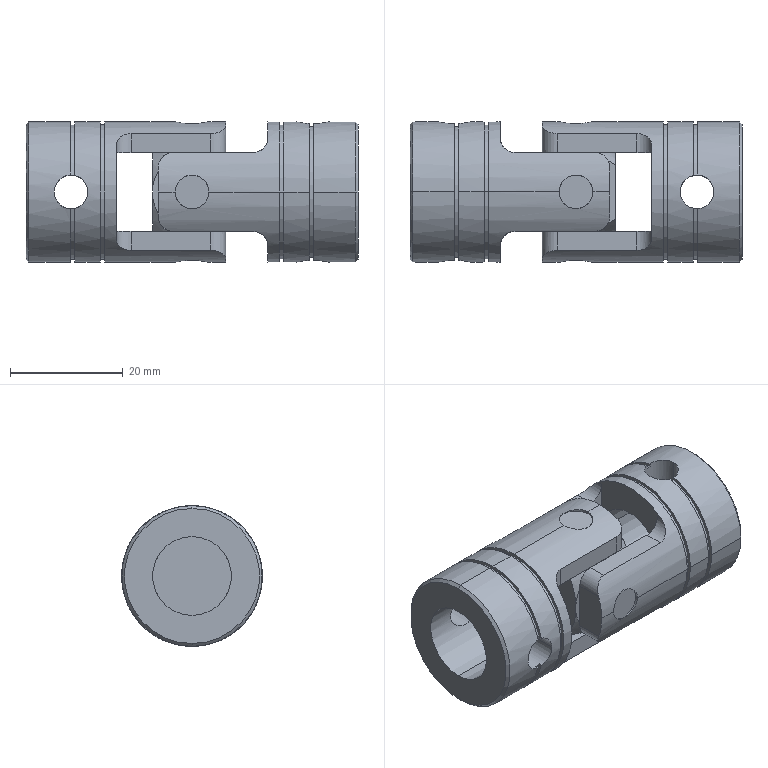Part | SolidWorks | features BaseBody 4 | 4 solids | 130 faces | box 59 x 25 x 25 mm | volume 17907 mm3 | cylinder 74 | plane 44 | spline 8 | cone 4 | commonest cylinder face diameters 6 x32 5.333 x16 25 x12 23.933 x10 14 x4